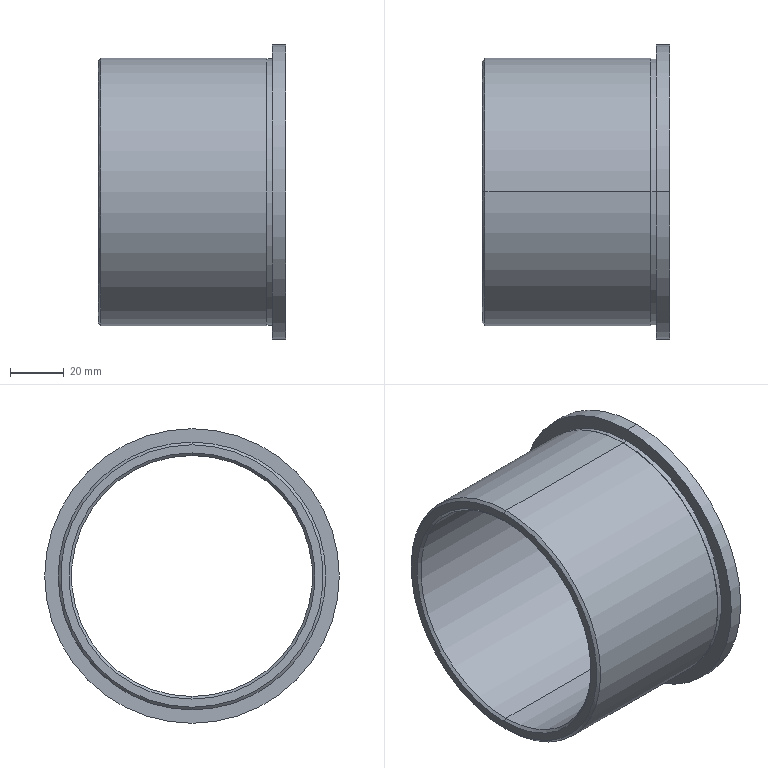Part | SolidWorks | features Revolution 1 | 1 solid | 18 faces | box 70 x 110 x 110 mm | volume 112148 mm3 | cylinder 8 | cone 6 | plane 4 | commonest cylinder face diameters 90 x2 99.6 x2 100 x2 110 x2
STEP:
#1=CARTESIAN_POINT('',(-35.,0.,49.));
#2=VERTEX_POINT('',#1);
#3=CARTESIAN_POINT('',(-35.,0.,-49.));
#4=VERTEX_POINT('',#3);
#5=CARTESIAN_POINT('',(-35.,0.,0.));
#6=DIRECTION('',(-1.,0.,0.));
#7=DIRECTION('',(0.,0.,1.));
#8=AXIS2_PLACEMENT_3D('',#5,#6,#7);
#9=CIRCLE('',#8,49.);
#10=EDGE_CURVE('',#2,#4,#9,.T.);
#11=ORIENTED_EDGE('',*,*,#10,.F.);
#12=CARTESIAN_POINT('',(-34.,0.,50.));
#13=VERTEX_POINT('',#12);
#14=CARTESIAN_POINT('',(-34.,0.,50.));
#15=DIRECTION('',(0.7071,0.,0.7071));
#16=VECTOR('',#15,1000.);
#17=LINE('',#14,#16);
#18=EDGE_CURVE('',#2,#13,#17,.T.);
#19=ORIENTED_EDGE('',*,*,#18,.T.);
#20=CARTESIAN_POINT('',(-34.,0.,-50.));
#21=VERTEX_POINT('',#20);
#22=CARTESIAN_POINT('',(-34.,0.,0.));
#23=DIRECTION('',(-1.,0.,0.));
#24=DIRECTION('',(0.,0.,1.));
#25=AXIS2_PLACEMENT_3D('',#22,#23,#24);
#26=CIRCLE('',#25,50.);
#27=EDGE_CURVE('',#13,#21,#26,.T.);
#28=ORIENTED_EDGE('',*,*,#27,.T.);
#29=CARTESIAN_POINT('',(-34.,0.,-50.));
#30=DIRECTION('',(0.7071,0.,-0.7071));
#31=VECTOR('',#30,1000.);
#32=LINE('',#29,#31);
#33=EDGE_CURVE('',#4,#21,#32,.T.);
#34=ORIENTED_EDGE('',*,*,#33,.F.);
#35=EDGE_LOOP('',(#11,#19,#28,#34));
#36=FACE_OUTER_BOUND('',#35,.T.);
#37=CARTESIAN_POINT('',(-34.,0.,0.));
#38=DIRECTION('',(1.,0.,0.));
#39=DIRECTION('',(0.,0.,-1.));
#40=AXIS2_PLACEMENT_3D('',#37,#38,#39);
#41=CONICAL_SURFACE('',#40,50.,0.7854);
#42=ADVANCED_FACE('',(#36),#41,.T.);
#43=CARTESIAN_POINT('',(28.,0.,50.));
#44=VERTEX_POINT('',#43);
#45=CARTESIAN_POINT('',(28.,0.,-50.));
#46=VERTEX_POINT('',#45);
#47=CARTESIAN_POINT('',(28.,0.,0.));
#48=DIRECTION('',(-1.,0.,0.));
#49=DIRECTION('',(0.,0.,1.));
#50=AXIS2_PLACEMENT_3D('',#47,#48,#49);
#51=CIRCLE('',#50,50.);
#52=EDGE_CURVE('',#44,#46,#51,.T.);
#53=ORIENTED_EDGE('',*,*,#52,.T.);
#54=CARTESIAN_POINT('',(-35.,0.,-50.));
#55=DIRECTION('',(-1.,0.,0.));
#56=VECTOR('',#55,1000.);
#57=LINE('',#54,#56);
#58=EDGE_CURVE('',#46,#21,#57,.T.);
#59=ORIENTED_EDGE('',*,*,#58,.T.);
#60=ORIENTED_EDGE('',*,*,#27,.F.);
#61=CARTESIAN_POINT('',(-35.,0.,50.));
#62=DIRECTION('',(-1.,0.,0.));
#63=VECTOR('',#62,1000.);
#64=LINE('',#61,#63);
#65=EDGE_CURVE('',#44,#13,#64,.T.);
#66=ORIENTED_EDGE('',*,*,#65,.F.);
#67=EDGE_LOOP('',(#53,#59,#60,#66));
#68=FACE_OUTER_BOUND('',#67,.T.);
#69=CARTESIAN_POINT('',(-35.,0.,0.));
#70=DIRECTION('',(-1.,0.,0.));
#71=DIRECTION('',(0.,0.,1.));
#72=AXIS2_PLACEMENT_3D('',#69,#70,#71);
#73=CYLINDRICAL_SURFACE('',#72,50.);
#74=ADVANCED_FACE('',(#68),#73,.T.);
#75=CARTESIAN_POINT('',(30.,0.,49.8));
#76=VERTEX_POINT('',#75);
#77=CARTESIAN_POINT('',(30.,0.,-49.8));
#78=VERTEX_POINT('',#77);
#79=CARTESIAN_POINT('',(30.,0.,0.));
#80=DIRECTION('',(-1.,0.,0.));
#81=DIRECTION('',(0.,0.,1.));
#82=AXIS2_PLACEMENT_3D('',#79,#80,#81);
#83=CIRCLE('',#82,49.8);
#84=EDGE_CURVE('',#76,#78,#83,.T.);
#85=ORIENTED_EDGE('',*,*,#84,.T.);
#86=CARTESIAN_POINT('',(28.,0.,-49.8));
#87=VERTEX_POINT('',#86);
#88=CARTESIAN_POINT('',(-35.,0.,-49.8));
#89=DIRECTION('',(-1.,0.,0.));
#90=VECTOR('',#89,1000.);
#91=LINE('',#88,#90);
#92=EDGE_CURVE('',#78,#87,#91,.T.);
#93=ORIENTED_EDGE('',*,*,#92,.T.);
#94=CARTESIAN_POINT('',(28.,0.,49.8));
#95=VERTEX_POINT('',#94);
#96=CARTESIAN_POINT('',(28.,0.,0.));
#97=DIRECTION('',(-1.,0.,0.));
#98=DIRECTION('',(0.,0.,1.));
#99=AXIS2_PLACEMENT_3D('',#96,#97,#98);
#100=CIRCLE('',#99,49.8);
#101=EDGE_CURVE('',#95,#87,#100,.T.);
#102=ORIENTED_EDGE('',*,*,#101,.F.);
#103=CARTESIAN_POINT('',(-35.,0.,49.8));
#104=DIRECTION('',(-1.,0.,0.));
#105=VECTOR('',#104,1000.);
#106=LINE('',#103,#105);
#107=EDGE_CURVE('',#76,#95,#106,.T.);
#108=ORIENTED_EDGE('',*,*,#107,.F.);
#109=EDGE_LOOP('',(#85,#93,#102,#108));
#110=FACE_OUTER_BOUND('',#109,.T.);
#111=CARTESIAN_POINT('',(-35.,0.,0.));
#112=DIRECTION('',(-1.,0.,0.));
#113=DIRECTION('',(0.,0.,1.));
#114=AXIS2_PLACEMENT_3D('',#111,#112,#113);
#115=CYLINDRICAL_SURFACE('',#114,49.8);
#116=ADVANCED_FACE('',(#110),#115,.T.);
#117=CARTESIAN_POINT('',(35.,0.,55.));
#118=VERTEX_POINT('',#117);
#119=CARTESIAN_POINT('',(35.,0.,-55.));
#120=VERTEX_POINT('',#119);
#121=CARTESIAN_POINT('',(35.,0.,0.));
#122=DIRECTION('',(-1.,0.,0.));
#123=DIRECTION('',(0.,0.,1.));
#124=AXIS2_PLACEMENT_3D('',#121,#122,#123);
#125=CIRCLE('',#124,55.);
#126=EDGE_CURVE('',#118,#120,#125,.T.);
#127=ORIENTED_EDGE('',*,*,#126,.T.);
#128=CARTESIAN_POINT('',(30.,0.,-55.));
#129=VERTEX_POINT('',#128);
#130=CARTESIAN_POINT('',(-35.,0.,-55.));
#131=DIRECTION('',(-1.,0.,0.));
#132=VECTOR('',#131,1000.);
#133=LINE('',#130,#132);
#134=EDGE_CURVE('',#120,#129,#133,.T.);
#135=ORIENTED_EDGE('',*,*,#134,.T.);
#136=CARTESIAN_POINT('',(30.,0.,55.));
#137=VERTEX_POINT('',#136);
#138=CARTESIAN_POINT('',(30.,0.,0.));
#139=DIRECTION('',(-1.,0.,0.));
#140=DIRECTION('',(0.,0.,1.));
#141=AXIS2_PLACEMENT_3D('',#138,#139,#140);
#142=CIRCLE('',#141,55.);
#143=EDGE_CURVE('',#137,#129,#142,.T.);
#144=ORIENTED_EDGE('',*,*,#143,.F.);
#145=CARTESIAN_POINT('',(-35.,0.,55.));
#146=DIRECTION('',(-1.,0.,0.));
#147=VECTOR('',#146,1000.);
#148=LINE('',#145,#147);
#149=EDGE_CURVE('',#118,#137,#148,.T.);
#150=ORIENTED_EDGE('',*,*,#149,.F.);
#151=EDGE_LOOP('',(#127,#135,#144,#150));
#152=FACE_OUTER_BOUND('',#151,.T.);
#153=CARTESIAN_POINT('',(-35.,0.,0.));
#154=DIRECTION('',(-1.,0.,0.));
#155=DIRECTION('',(0.,0.,1.));
#156=AXIS2_PLACEMENT_3D('',#153,#154,#155);
#157=CYLINDRICAL_SURFACE('',#156,55.);
#158=ADVANCED_FACE('',(#152),#157,.T.);
#159=CARTESIAN_POINT('',(34.,0.,-45.));
#160=VERTEX_POINT('',#159);
#161=CARTESIAN_POINT('',(34.,0.,45.));
#162=VERTEX_POINT('',#161);
#163=CARTESIAN_POINT('',(34.,0.,0.));
#164=DIRECTION('',(-1.,0.,0.));
#165=DIRECTION('',(0.,0.,1.));
#166=AXIS2_PLACEMENT_3D('',#163,#164,#165);
#167=CIRCLE('',#166,45.);
#168=EDGE_CURVE('',#160,#162,#167,.T.);
#169=ORIENTED_EDGE('',*,*,#168,.T.);
#170=CARTESIAN_POINT('',(35.,0.,45.966));
#171=VERTEX_POINT('',#170);
#172=CARTESIAN_POINT('',(34.,0.,45.));
#173=DIRECTION('',(0.7193,0.,0.6947));
#174=VECTOR('',#173,1000.);
#175=LINE('',#172,#174);
#176=EDGE_CURVE('',#162,#171,#175,.T.);
#177=ORIENTED_EDGE('',*,*,#176,.T.);
#178=CARTESIAN_POINT('',(35.,0.,-45.966));
#179=VERTEX_POINT('',#178);
#180=CARTESIAN_POINT('',(35.,0.,0.));
#181=DIRECTION('',(-1.,0.,0.));
#182=DIRECTION('',(0.,0.,1.));
#183=AXIS2_PLACEMENT_3D('',#180,#181,#182);
#184=CIRCLE('',#183,45.966);
#185=EDGE_CURVE('',#179,#171,#184,.T.);
#186=ORIENTED_EDGE('',*,*,#185,.F.);
#187=CARTESIAN_POINT('',(34.,0.,-45.));
#188=DIRECTION('',(0.7193,0.,-0.6947));
#189=VECTOR('',#188,1000.);
#190=LINE('',#187,#189);
#191=EDGE_CURVE('',#160,#179,#190,.T.);
#192=ORIENTED_EDGE('',*,*,#191,.F.);
#193=EDGE_LOOP('',(#169,#177,#186,#192));
#194=FACE_OUTER_BOUND('',#193,.T.);
#195=CARTESIAN_POINT('',(34.,0.,0.));
#196=DIRECTION('',(1.,0.,0.));
#197=DIRECTION('',(0.,0.,-1.));
#198=AXIS2_PLACEMENT_3D('',#195,#196,#197);
#199=CONICAL_SURFACE('',#198,45.,0.7679);
#200=ADVANCED_FACE('',(#194),#199,.F.);
#201=ORIENTED_EDGE('',*,*,#168,.F.);
#202=CARTESIAN_POINT('',(-34.,0.,-45.));
#203=VERTEX_POINT('',#202);
#204=CARTESIAN_POINT('',(-35.,0.,-45.));
#205=DIRECTION('',(-1.,0.,0.));
#206=VECTOR('',#205,1000.);
#207=LINE('',#204,#206);
#208=EDGE_CURVE('',#160,#203,#207,.T.);
#209=ORIENTED_EDGE('',*,*,#208,.T.);
#210=CARTESIAN_POINT('',(-34.,0.,45.));
#211=VERTEX_POINT('',#210);
#212=CARTESIAN_POINT('',(-34.,0.,0.));
#213=DIRECTION('',(-1.,0.,0.));
#214=DIRECTION('',(0.,0.,1.));
#215=AXIS2_PLACEMENT_3D('',#212,#213,#214);
#216=CIRCLE('',#215,45.);
#217=EDGE_CURVE('',#203,#211,#216,.T.);
#218=ORIENTED_EDGE('',*,*,#217,.T.);
#219=CARTESIAN_POINT('',(-35.,0.,45.));
#220=DIRECTION('',(-1.,0.,0.));
#221=VECTOR('',#220,1000.);
#222=LINE('',#219,#221);
#223=EDGE_CURVE('',#162,#211,#222,.T.);
#224=ORIENTED_EDGE('',*,*,#223,.F.);
#225=EDGE_LOOP('',(#201,#209,#218,#224));
#226=FACE_OUTER_BOUND('',#225,.T.);
#227=CARTESIAN_POINT('',(-35.,0.,0.));
#228=DIRECTION('',(-1.,0.,0.));
#229=DIRECTION('',(0.,0.,1.));
#230=AXIS2_PLACEMENT_3D('',#227,#228,#229);
#231=CYLINDRICAL_SURFACE('',#230,45.);
#232=ADVANCED_FACE('',(#226),#231,.F.);
#233=ORIENTED_EDGE('',*,*,#217,.F.);
#234=CARTESIAN_POINT('',(-35.,0.,-45.966));
#235=VERTEX_POINT('',#234);
#236=CARTESIAN_POINT('',(-35.,0.,-45.966));
#237=DIRECTION('',(-0.7193,0.,-0.6947));
#238=VECTOR('',#237,1000.);
#239=LINE('',#236,#238);
#240=EDGE_CURVE('',#203,#235,#239,.T.);
#241=ORIENTED_EDGE('',*,*,#240,.T.);
#242=CARTESIAN_POINT('',(-35.,0.,45.966));
#243=VERTEX_POINT('',#242);
#244=CARTESIAN_POINT('',(-35.,0.,0.));
#245=DIRECTION('',(-1.,0.,0.));
#246=DIRECTION('',(0.,0.,1.));
#247=AXIS2_PLACEMENT_3D('',#244,#245,#246);
#248=CIRCLE('',#247,45.966);
#249=EDGE_CURVE('',#235,#243,#248,.T.);
#250=ORIENTED_EDGE('',*,*,#249,.T.);
#251=CARTESIAN_POINT('',(-35.,0.,45.966));
#252=DIRECTION('',(-0.7193,0.,0.6947));
#253=VECTOR('',#252,1000.);
#254=LINE('',#251,#253);
#255=EDGE_CURVE('',#211,#243,#254,.T.);
#256=ORIENTED_EDGE('',*,*,#255,.F.);
#257=EDGE_LOOP('',(#233,#241,#250,#256));
#258=FACE_OUTER_BOUND('',#257,.T.);
#259=CARTESIAN_POINT('',(-35.,0.,0.));
#260=DIRECTION('',(-1.,0.,0.));
#261=DIRECTION('',(0.,0.,1.));
#262=AXIS2_PLACEMENT_3D('',#259,#260,#261);
#263=CONICAL_SURFACE('',#262,45.966,0.7679);
#264=ADVANCED_FACE('',(#258),#263,.F.);
#265=CARTESIAN_POINT('',(-35.,0.,0.));
#266=DIRECTION('',(-1.,0.,0.));
#267=DIRECTION('',(0.,0.,1.));
#268=AXIS2_PLACEMENT_3D('',#265,#266,#267);
#269=CIRCLE('',#268,45.966);
#270=EDGE_CURVE('',#243,#235,#269,.T.);
#271=ORIENTED_EDGE('',*,*,#270,.F.);
#272=ORIENTED_EDGE('',*,*,#249,.F.);
#273=EDGE_LOOP('',(#271,#272));
#274=FACE_BOUND('',#273,.T.);
#275=CARTESIAN_POINT('',(-35.,0.,0.));
#276=DIRECTION('',(-1.,0.,0.));
#277=DIRECTION('',(0.,0.,1.));
#278=AXIS2_PLACEMENT_3D('',#275,#276,#277);
#279=CIRCLE('',#278,49.);
#280=EDGE_CURVE('',#4,#2,#279,.T.);
#281=ORIENTED_EDGE('',*,*,#280,.T.);
#282=ORIENTED_EDGE('',*,*,#10,.T.);
#283=EDGE_LOOP('',(#281,#282));
#284=FACE_OUTER_BOUND('',#283,.T.);
#285=CARTESIAN_POINT('',(-35.,49.,0.));
#286=DIRECTION('',(1.,0.,0.));
#287=DIRECTION('',(0.,0.,-1.));
#288=AXIS2_PLACEMENT_3D('',#285,#286,#287);
#289=PLANE('',#288);
#290=ADVANCED_FACE('',(#274,#284),#289,.F.);
#291=ORIENTED_EDGE('',*,*,#240,.F.);
#292=CARTESIAN_POINT('',(-34.,0.,0.));
#293=DIRECTION('',(-1.,0.,0.));
#294=DIRECTION('',(0.,0.,1.));
#295=AXIS2_PLACEMENT_3D('',#292,#293,#294);
#296=CIRCLE('',#295,45.);
#297=EDGE_CURVE('',#211,#203,#296,.T.);
#298=ORIENTED_EDGE('',*,*,#297,.F.);
#299=ORIENTED_EDGE('',*,*,#255,.T.);
#300=ORIENTED_EDGE('',*,*,#270,.T.);
#301=EDGE_LOOP('',(#291,#298,#299,#300));
#302=FACE_OUTER_BOUND('',#301,.T.);
#303=CARTESIAN_POINT('',(-35.,0.,0.));
#304=DIRECTION('',(-1.,0.,0.));
#305=DIRECTION('',(0.,0.,1.));
#306=AXIS2_PLACEMENT_3D('',#303,#304,#305);
#307=CONICAL_SURFACE('',#306,45.966,0.7679);
#308=ADVANCED_FACE('',(#302),#307,.F.);
#309=ORIENTED_EDGE('',*,*,#208,.F.);
#310=CARTESIAN_POINT('',(34.,0.,0.));
#311=DIRECTION('',(-1.,0.,0.));
#312=DIRECTION('',(0.,0.,1.));
#313=AXIS2_PLACEMENT_3D('',#310,#311,#312);
#314=CIRCLE('',#313,45.);
#315=EDGE_CURVE('',#162,#160,#314,.T.);
#316=ORIENTED_EDGE('',*,*,#315,.F.);
#317=ORIENTED_EDGE('',*,*,#223,.T.);
#318=ORIENTED_EDGE('',*,*,#297,.T.);
#319=EDGE_LOOP('',(#309,#316,#317,#318));
#320=FACE_OUTER_BOUND('',#319,.T.);
#321=CARTESIAN_POINT('',(-35.,0.,0.));
#322=DIRECTION('',(-1.,0.,0.));
#323=DIRECTION('',(0.,0.,1.));
#324=AXIS2_PLACEMENT_3D('',#321,#322,#323);
#325=CYLINDRICAL_SURFACE('',#324,45.);
#326=ADVANCED_FACE('',(#320),#325,.F.);
#327=ORIENTED_EDGE('',*,*,#176,.F.);
#328=ORIENTED_EDGE('',*,*,#315,.T.);
#329=ORIENTED_EDGE('',*,*,#191,.T.);
#330=CARTESIAN_POINT('',(35.,0.,0.));
#331=DIRECTION('',(-1.,0.,0.));
#332=DIRECTION('',(0.,0.,1.));
#333=AXIS2_PLACEMENT_3D('',#330,#331,#332);
#334=CIRCLE('',#333,45.966);
#335=EDGE_CURVE('',#171,#179,#334,.T.);
#336=ORIENTED_EDGE('',*,*,#335,.F.);
#337=EDGE_LOOP('',(#327,#328,#329,#336));
#338=FACE_OUTER_BOUND('',#337,.T.);
#339=CARTESIAN_POINT('',(34.,0.,0.));
#340=DIRECTION('',(1.,0.,0.));
#341=DIRECTION('',(0.,0.,-1.));
#342=AXIS2_PLACEMENT_3D('',#339,#340,#341);
#343=CONICAL_SURFACE('',#342,45.,0.7679);
#344=ADVANCED_FACE('',(#338),#343,.F.);
#345=ORIENTED_EDGE('',*,*,#126,.F.);
#346=CARTESIAN_POINT('',(35.,0.,0.));
#347=DIRECTION('',(-1.,0.,0.));
#348=DIRECTION('',(0.,0.,1.));
#349=AXIS2_PLACEMENT_3D('',#346,#347,#348);
#350=CIRCLE('',#349,55.);
#351=EDGE_CURVE('',#120,#118,#350,.T.);
#352=ORIENTED_EDGE('',*,*,#351,.F.);
#353=EDGE_LOOP('',(#345,#352));
#354=FACE_OUTER_BOUND('',#353,.T.);
#355=ORIENTED_EDGE('',*,*,#185,.T.);
#356=ORIENTED_EDGE('',*,*,#335,.T.);
#357=EDGE_LOOP('',(#355,#356));
#358=FACE_BOUND('',#357,.T.);
#359=CARTESIAN_POINT('',(35.,45.966,0.));
#360=DIRECTION('',(-1.,0.,0.));
#361=DIRECTION('',(0.,0.,1.));
#362=AXIS2_PLACEMENT_3D('',#359,#360,#361);
#363=PLANE('',#362);
#364=ADVANCED_FACE('',(#354,#358),#363,.F.);
#365=ORIENTED_EDGE('',*,*,#134,.F.);
#366=ORIENTED_EDGE('',*,*,#351,.T.);
#367=ORIENTED_EDGE('',*,*,#149,.T.);
#368=CARTESIAN_POINT('',(30.,0.,0.));
#369=DIRECTION('',(-1.,0.,0.));
#370=DIRECTION('',(0.,0.,1.));
#371=AXIS2_PLACEMENT_3D('',#368,#369,#370);
#372=CIRCLE('',#371,55.);
#373=EDGE_CURVE('',#129,#137,#372,.T.);
#374=ORIENTED_EDGE('',*,*,#373,.F.);
#375=EDGE_LOOP('',(#365,#366,#367,#374));
#376=FACE_OUTER_BOUND('',#375,.T.);
#377=CARTESIAN_POINT('',(-35.,0.,0.));
#378=DIRECTION('',(-1.,0.,0.));
#379=DIRECTION('',(0.,0.,1.));
#380=AXIS2_PLACEMENT_3D('',#377,#378,#379);
#381=CYLINDRICAL_SURFACE('',#380,55.);
#382=ADVANCED_FACE('',(#376),#381,.T.);
#383=ORIENTED_EDGE('',*,*,#84,.F.);
#384=CARTESIAN_POINT('',(30.,0.,0.));
#385=DIRECTION('',(-1.,0.,0.));
#386=DIRECTION('',(0.,0.,1.));
#387=AXIS2_PLACEMENT_3D('',#384,#385,#386);
#388=CIRCLE('',#387,49.8);
#389=EDGE_CURVE('',#78,#76,#388,.T.);
#390=ORIENTED_EDGE('',*,*,#389,.F.);
#391=EDGE_LOOP('',(#383,#390));
#392=FACE_BOUND('',#391,.T.);
#393=ORIENTED_EDGE('',*,*,#143,.T.);
#394=ORIENTED_EDGE('',*,*,#373,.T.);
#395=EDGE_LOOP('',(#393,#394));
#396=FACE_OUTER_BOUND('',#395,.T.);
#397=CARTESIAN_POINT('',(30.,55.,0.));
#398=DIRECTION('',(1.,0.,0.));
#399=DIRECTION('',(0.,0.,-1.));
#400=AXIS2_PLACEMENT_3D('',#397,#398,#399);
#401=PLANE('',#400);
#402=ADVANCED_FACE('',(#392,#396),#401,.F.);
#403=ORIENTED_EDGE('',*,*,#92,.F.);
#404=ORIENTED_EDGE('',*,*,#389,.T.);
#405=ORIENTED_EDGE('',*,*,#107,.T.);
#406=CARTESIAN_POINT('',(28.,0.,0.));
#407=DIRECTION('',(-1.,0.,0.));
#408=DIRECTION('',(0.,0.,1.));
#409=AXIS2_PLACEMENT_3D('',#406,#407,#408);
#410=CIRCLE('',#409,49.8);
#411=EDGE_CURVE('',#87,#95,#410,.T.);
#412=ORIENTED_EDGE('',*,*,#411,.F.);
#413=EDGE_LOOP('',(#403,#404,#405,#412));
#414=FACE_OUTER_BOUND('',#413,.T.);
#415=CARTESIAN_POINT('',(-35.,0.,0.));
#416=DIRECTION('',(-1.,0.,0.));
#417=DIRECTION('',(0.,0.,1.));
#418=AXIS2_PLACEMENT_3D('',#415,#416,#417);
#419=CYLINDRICAL_SURFACE('',#418,49.8);
#420=ADVANCED_FACE('',(#414),#419,.T.);
#421=ORIENTED_EDGE('',*,*,#52,.F.);
#422=CARTESIAN_POINT('',(28.,0.,0.));
#423=DIRECTION('',(-1.,0.,0.));
#424=DIRECTION('',(0.,0.,1.));
#425=AXIS2_PLACEMENT_3D('',#422,#423,#424);
#426=CIRCLE('',#425,50.);
#427=EDGE_CURVE('',#46,#44,#426,.T.);
#428=ORIENTED_EDGE('',*,*,#427,.F.);
#429=EDGE_LOOP('',(#421,#428));
#430=FACE_OUTER_BOUND('',#429,.T.);
#431=ORIENTED_EDGE('',*,*,#101,.T.);
#432=ORIENTED_EDGE('',*,*,#411,.T.);
#433=EDGE_LOOP('',(#431,#432));
#434=FACE_BOUND('',#433,.T.);
#435=CARTESIAN_POINT('',(28.,49.8,0.));
#436=DIRECTION('',(-1.,0.,0.));
#437=DIRECTION('',(0.,0.,1.));
#438=AXIS2_PLACEMENT_3D('',#435,#436,#437);
#439=PLANE('',#438);
#440=ADVANCED_FACE('',(#430,#434),#439,.F.);
#441=ORIENTED_EDGE('',*,*,#58,.F.);
#442=ORIENTED_EDGE('',*,*,#427,.T.);
#443=ORIENTED_EDGE('',*,*,#65,.T.);
#444=CARTESIAN_POINT('',(-34.,0.,0.));
#445=DIRECTION('',(-1.,0.,0.));
#446=DIRECTION('',(0.,0.,1.));
#447=AXIS2_PLACEMENT_3D('',#444,#445,#446);
#448=CIRCLE('',#447,50.);
#449=EDGE_CURVE('',#21,#13,#448,.T.);
#450=ORIENTED_EDGE('',*,*,#449,.F.);
#451=EDGE_LOOP('',(#441,#442,#443,#450));
#452=FACE_OUTER_BOUND('',#451,.T.);
#453=CARTESIAN_POINT('',(-35.,0.,0.));
#454=DIRECTION('',(-1.,0.,0.));
#455=DIRECTION('',(0.,0.,1.));
#456=AXIS2_PLACEMENT_3D('',#453,#454,#455);
#457=CYLINDRICAL_SURFACE('',#456,50.);
#458=ADVANCED_FACE('',(#452),#457,.T.);
#459=ORIENTED_EDGE('',*,*,#18,.F.);
#460=ORIENTED_EDGE('',*,*,#280,.F.);
#461=ORIENTED_EDGE('',*,*,#33,.T.);
#462=ORIENTED_EDGE('',*,*,#449,.T.);
#463=EDGE_LOOP('',(#459,#460,#461,#462));
#464=FACE_OUTER_BOUND('',#463,.T.);
#465=CARTESIAN_POINT('',(-34.,0.,0.));
#466=DIRECTION('',(1.,0.,0.));
#467=DIRECTION('',(0.,0.,-1.));
#468=AXIS2_PLACEMENT_3D('',#465,#466,#467);
#469=CONICAL_SURFACE('',#468,50.,0.7854);
#470=ADVANCED_FACE('',(#464),#469,.T.);
#471=CLOSED_SHELL('',(#42,#74,#116,#158,#200,#232,#264,#290,#308,#326,#344,#364,#382,#402,#420,#440,#458,#470));
#472=MANIFOLD_SOLID_BREP('',#471);
#473=CARTESIAN_POINT('',(0.,0.,0.));
#474=DIRECTION('',(0.,0.,1.));
#475=DIRECTION('',(1.,0.,0.));
#476=AXIS2_PLACEMENT_3D('',#473,#474,#475);
#477=(LENGTH_UNIT()NAMED_UNIT(*)SI_UNIT(.MILLI.,.METRE.));
#478=UNCERTAINTY_MEASURE_WITH_UNIT(LENGTH_MEASURE(0.00001),#477,'','');
#479=(NAMED_UNIT(*)PLANE_ANGLE_UNIT()SI_UNIT($,.RADIAN.));
#480=(NAMED_UNIT(*)SI_UNIT($,.STERADIAN.)SOLID_ANGLE_UNIT());
#481=(GEOMETRIC_REPRESENTATION_CONTEXT(3)GLOBAL_UNCERTAINTY_ASSIGNED_CONTEXT((#478))GLOBAL_UNIT_ASSIGNED_CONTEXT((#477,#479,#480))REPRESENTATION_CONTEXT('',''));
#482=ADVANCED_BREP_SHAPE_REPRESENTATION('',(#472,#476),#481);